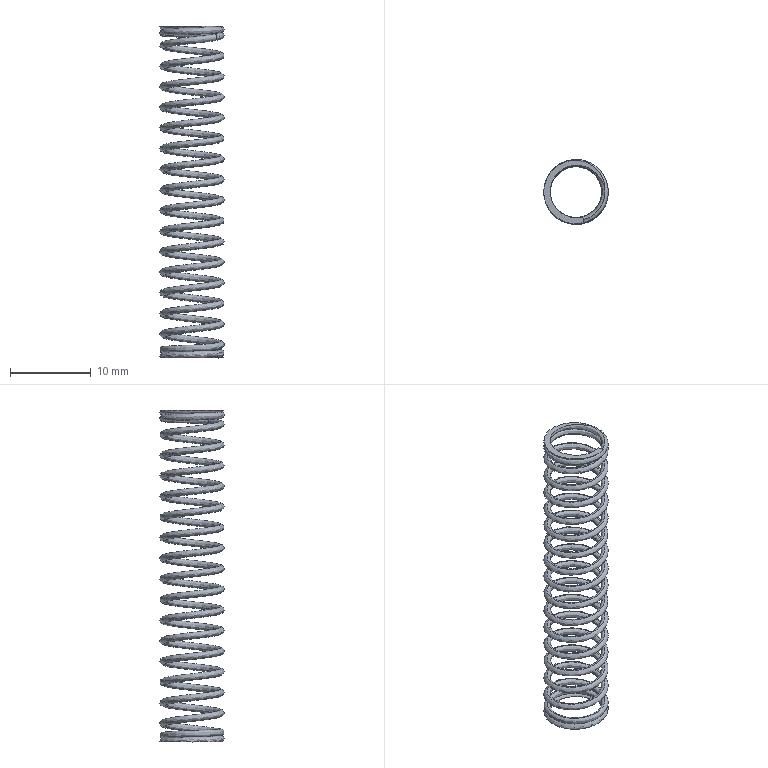Part | NX | features BREP 1 | 1 solid | 8 faces | volume 204.552 mm3 | plane 4 | spline 4